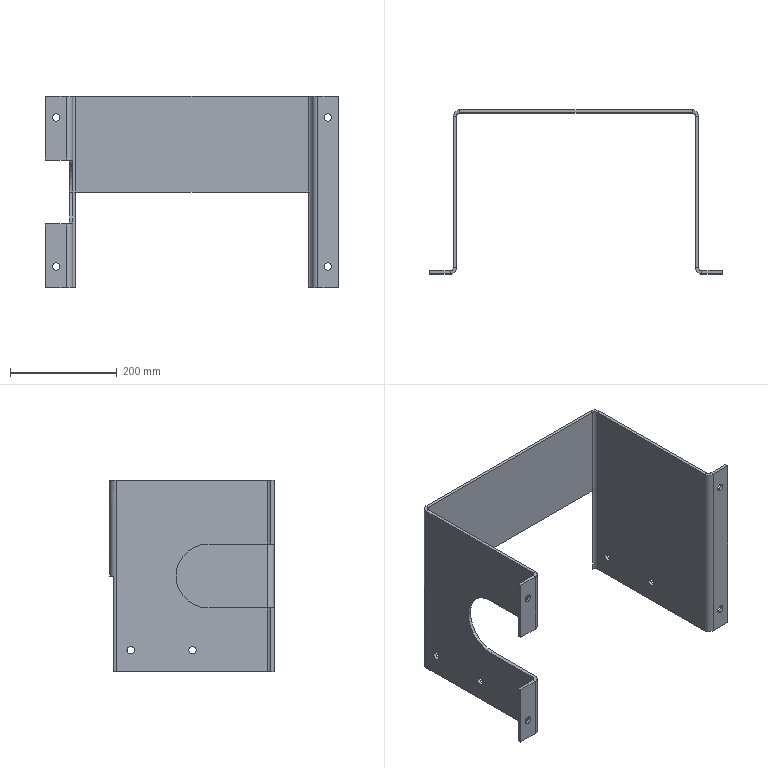Part | STEP file | Anti-jump chain fixing seat | 1 solid | 65 faces | box 550 x 308 x 360 mm | volume 1812248 mm3 | plane 37 | cylinder 28 | commonest cylinder face diameters 14 x16 12 x5 24 x5 120 x2